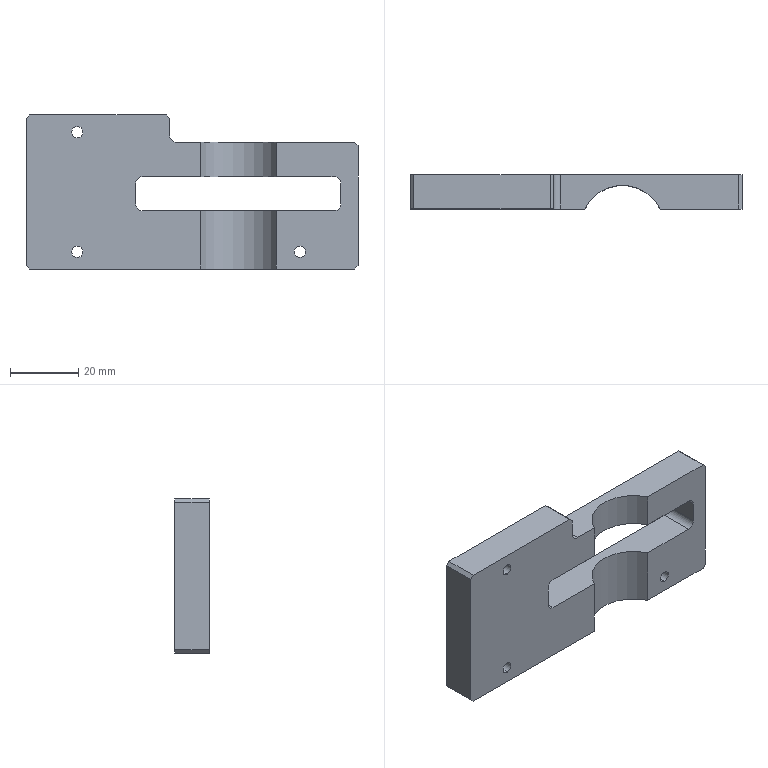Part | SolidWorks | features ICE 9, 3DProfileFeature 2, Fillet 2, HoleWzd 2, Chamfer 1, Extrusion 1 | 1 solid | 39 faces | box 97 x 10 x 45 mm | volume 29685 mm3 | plane 18 | cylinder 17 | cone 4 | commonest cylinder face diameters 3.3 x6 4 x5 4.2 x4 24.5 x2
STEP:
#1=CARTESIAN_POINT('',(-152.,0.,-19.15));
#2=VERTEX_POINT('',#1);
#3=CARTESIAN_POINT('',(-152.,0.,-15.85));
#4=VERTEX_POINT('',#3);
#5=CARTESIAN_POINT('',(-152.,0.,-17.5));
#6=DIRECTION('',(0.,1.,0.));
#7=DIRECTION('',(0.,0.,1.));
#8=AXIS2_PLACEMENT_3D('',#5,#6,#7);
#9=CIRCLE('',#8,1.65);
#10=EDGE_CURVE('',#2,#4,#9,.T.);
#11=ORIENTED_EDGE('',*,*,#10,.F.);
#12=CARTESIAN_POINT('',(-152.,10.,-19.15));
#13=VERTEX_POINT('',#12);
#14=CARTESIAN_POINT('',(-152.,10.,-19.15));
#15=DIRECTION('',(0.,1.,0.));
#16=VECTOR('',#15,1000.);
#17=LINE('',#14,#16);
#18=EDGE_CURVE('',#2,#13,#17,.T.);
#19=ORIENTED_EDGE('',*,*,#18,.T.);
#20=CARTESIAN_POINT('',(-152.,10.,-15.85));
#21=VERTEX_POINT('',#20);
#22=CARTESIAN_POINT('',(-152.,10.,-17.5));
#23=DIRECTION('',(0.,1.,0.));
#24=DIRECTION('',(0.,0.,1.));
#25=AXIS2_PLACEMENT_3D('',#22,#23,#24);
#26=CIRCLE('',#25,1.65);
#27=EDGE_CURVE('',#13,#21,#26,.T.);
#28=ORIENTED_EDGE('',*,*,#27,.T.);
#29=CARTESIAN_POINT('',(-152.,10.,-15.85));
#30=DIRECTION('',(0.,1.,0.));
#31=VECTOR('',#30,1000.);
#32=LINE('',#29,#31);
#33=EDGE_CURVE('',#4,#21,#32,.T.);
#34=ORIENTED_EDGE('',*,*,#33,.F.);
#35=EDGE_LOOP('',(#11,#19,#28,#34));
#36=FACE_OUTER_BOUND('',#35,.T.);
#37=CARTESIAN_POINT('',(-152.,10.,-17.5));
#38=DIRECTION('',(0.,1.,0.));
#39=DIRECTION('',(0.,0.,1.));
#40=AXIS2_PLACEMENT_3D('',#37,#38,#39);
#41=CYLINDRICAL_SURFACE('',#40,1.65);
#42=ADVANCED_FACE('',(#36),#41,.F.);
#43=CARTESIAN_POINT('',(-87.,0.,-19.15));
#44=VERTEX_POINT('',#43);
#45=CARTESIAN_POINT('',(-87.,0.,-15.85));
#46=VERTEX_POINT('',#45);
#47=CARTESIAN_POINT('',(-87.,0.,-17.5));
#48=DIRECTION('',(0.,1.,0.));
#49=DIRECTION('',(0.,0.,1.));
#50=AXIS2_PLACEMENT_3D('',#47,#48,#49);
#51=CIRCLE('',#50,1.65);
#52=EDGE_CURVE('',#44,#46,#51,.T.);
#53=ORIENTED_EDGE('',*,*,#52,.F.);
#54=CARTESIAN_POINT('',(-87.,10.,-19.15));
#55=VERTEX_POINT('',#54);
#56=CARTESIAN_POINT('',(-87.,10.,-19.15));
#57=DIRECTION('',(0.,1.,0.));
#58=VECTOR('',#57,1000.);
#59=LINE('',#56,#58);
#60=EDGE_CURVE('',#44,#55,#59,.T.);
#61=ORIENTED_EDGE('',*,*,#60,.T.);
#62=CARTESIAN_POINT('',(-87.,10.,-15.85));
#63=VERTEX_POINT('',#62);
#64=CARTESIAN_POINT('',(-87.,10.,-17.5));
#65=DIRECTION('',(0.,1.,0.));
#66=DIRECTION('',(0.,0.,1.));
#67=AXIS2_PLACEMENT_3D('',#64,#65,#66);
#68=CIRCLE('',#67,1.65);
#69=EDGE_CURVE('',#55,#63,#68,.T.);
#70=ORIENTED_EDGE('',*,*,#69,.T.);
#71=CARTESIAN_POINT('',(-87.,10.,-15.85));
#72=DIRECTION('',(0.,1.,0.));
#73=VECTOR('',#72,1000.);
#74=LINE('',#71,#73);
#75=EDGE_CURVE('',#46,#63,#74,.T.);
#76=ORIENTED_EDGE('',*,*,#75,.F.);
#77=EDGE_LOOP('',(#53,#61,#70,#76));
#78=FACE_OUTER_BOUND('',#77,.T.);
#79=CARTESIAN_POINT('',(-87.,10.,-17.5));
#80=DIRECTION('',(0.,1.,0.));
#81=DIRECTION('',(0.,0.,1.));
#82=AXIS2_PLACEMENT_3D('',#79,#80,#81);
#83=CYLINDRICAL_SURFACE('',#82,1.65);
#84=ADVANCED_FACE('',(#78),#83,.F.);
#85=CARTESIAN_POINT('',(-152.,0.,15.85));
#86=VERTEX_POINT('',#85);
#87=CARTESIAN_POINT('',(-152.,0.,19.15));
#88=VERTEX_POINT('',#87);
#89=CARTESIAN_POINT('',(-152.,0.,17.5));
#90=DIRECTION('',(0.,1.,0.));
#91=DIRECTION('',(0.,0.,1.));
#92=AXIS2_PLACEMENT_3D('',#89,#90,#91);
#93=CIRCLE('',#92,1.65);
#94=EDGE_CURVE('',#86,#88,#93,.T.);
#95=ORIENTED_EDGE('',*,*,#94,.F.);
#96=CARTESIAN_POINT('',(-152.,10.,15.85));
#97=VERTEX_POINT('',#96);
#98=CARTESIAN_POINT('',(-152.,10.,15.85));
#99=DIRECTION('',(0.,1.,0.));
#100=VECTOR('',#99,1000.);
#101=LINE('',#98,#100);
#102=EDGE_CURVE('',#86,#97,#101,.T.);
#103=ORIENTED_EDGE('',*,*,#102,.T.);
#104=CARTESIAN_POINT('',(-152.,10.,19.15));
#105=VERTEX_POINT('',#104);
#106=CARTESIAN_POINT('',(-152.,10.,17.5));
#107=DIRECTION('',(0.,1.,0.));
#108=DIRECTION('',(0.,0.,1.));
#109=AXIS2_PLACEMENT_3D('',#106,#107,#108);
#110=CIRCLE('',#109,1.65);
#111=EDGE_CURVE('',#97,#105,#110,.T.);
#112=ORIENTED_EDGE('',*,*,#111,.T.);
#113=CARTESIAN_POINT('',(-152.,10.,19.15));
#114=DIRECTION('',(0.,1.,0.));
#115=VECTOR('',#114,1000.);
#116=LINE('',#113,#115);
#117=EDGE_CURVE('',#88,#105,#116,.T.);
#118=ORIENTED_EDGE('',*,*,#117,.F.);
#119=EDGE_LOOP('',(#95,#103,#112,#118));
#120=FACE_OUTER_BOUND('',#119,.T.);
#121=CARTESIAN_POINT('',(-152.,10.,17.5));
#122=DIRECTION('',(0.,1.,0.));
#123=DIRECTION('',(0.,0.,1.));
#124=AXIS2_PLACEMENT_3D('',#121,#122,#123);
#125=CYLINDRICAL_SURFACE('',#124,1.65);
#126=ADVANCED_FACE('',(#120),#125,.F.);
#127=CARTESIAN_POINT('',(-156.9,5.,-10.1));
#128=VERTEX_POINT('',#127);
#129=CARTESIAN_POINT('',(-161.1,5.,-10.1));
#130=VERTEX_POINT('',#129);
#131=CARTESIAN_POINT('',(-159.,5.,-10.1));
#132=DIRECTION('',(0.,0.,-1.));
#133=DIRECTION('',(-1.,0.,0.));
#134=AXIS2_PLACEMENT_3D('',#131,#132,#133);
#135=CIRCLE('',#134,2.1);
#136=EDGE_CURVE('',#128,#130,#135,.T.);
#137=ORIENTED_EDGE('',*,*,#136,.F.);
#138=CARTESIAN_POINT('',(-156.9,5.,-22.5));
#139=VERTEX_POINT('',#138);
#140=CARTESIAN_POINT('',(-156.9,5.,-22.5));
#141=DIRECTION('',(0.,0.,-1.));
#142=VECTOR('',#141,1000.);
#143=LINE('',#140,#142);
#144=EDGE_CURVE('',#128,#139,#143,.T.);
#145=ORIENTED_EDGE('',*,*,#144,.T.);
#146=CARTESIAN_POINT('',(-161.1,5.,-22.5));
#147=VERTEX_POINT('',#146);
#148=CARTESIAN_POINT('',(-159.,5.,-22.5));
#149=DIRECTION('',(0.,0.,-1.));
#150=DIRECTION('',(-1.,0.,0.));
#151=AXIS2_PLACEMENT_3D('',#148,#149,#150);
#152=CIRCLE('',#151,2.1);
#153=EDGE_CURVE('',#139,#147,#152,.T.);
#154=ORIENTED_EDGE('',*,*,#153,.T.);
#155=CARTESIAN_POINT('',(-161.1,5.,-22.5));
#156=DIRECTION('',(0.,0.,-1.));
#157=VECTOR('',#156,1000.);
#158=LINE('',#155,#157);
#159=EDGE_CURVE('',#130,#147,#158,.T.);
#160=ORIENTED_EDGE('',*,*,#159,.F.);
#161=EDGE_LOOP('',(#137,#145,#154,#160));
#162=FACE_OUTER_BOUND('',#161,.T.);
#163=CARTESIAN_POINT('',(-159.,5.,-22.5));
#164=DIRECTION('',(0.,0.,-1.));
#165=DIRECTION('',(-1.,0.,0.));
#166=AXIS2_PLACEMENT_3D('',#163,#164,#165);
#167=CYLINDRICAL_SURFACE('',#166,2.1);
#168=ADVANCED_FACE('',(#162),#167,.F.);
#169=CARTESIAN_POINT('',(-159.,5.,-8.838));
#170=VERTEX_POINT('',#169);
#171=CARTESIAN_POINT('',(-161.1,5.,-10.1));
#172=DIRECTION('',(-0.8572,0.,-0.515));
#173=VECTOR('',#172,1000.);
#174=LINE('',#171,#173);
#175=EDGE_CURVE('',#170,#130,#174,.T.);
#176=ORIENTED_EDGE('',*,*,#175,.F.);
#177=CARTESIAN_POINT('',(-156.9,5.,-10.1));
#178=DIRECTION('',(0.8572,0.,-0.515));
#179=VECTOR('',#178,1000.);
#180=LINE('',#177,#179);
#181=EDGE_CURVE('',#170,#128,#180,.T.);
#182=ORIENTED_EDGE('',*,*,#181,.T.);
#183=ORIENTED_EDGE('',*,*,#136,.T.);
#184=EDGE_LOOP('',(#176,#182,#183));
#185=FACE_OUTER_BOUND('',#184,.T.);
#186=CARTESIAN_POINT('',(-159.,5.,-10.1));
#187=DIRECTION('',(0.,0.,-1.));
#188=DIRECTION('',(-1.,0.,0.));
#189=AXIS2_PLACEMENT_3D('',#186,#187,#188);
#190=CONICAL_SURFACE('',#189,2.1,1.03);
#191=ADVANCED_FACE('',(#185),#190,.F.);
#192=CARTESIAN_POINT('',(-78.9,5.,-10.1));
#193=VERTEX_POINT('',#192);
#194=CARTESIAN_POINT('',(-83.1,5.,-10.1));
#195=VERTEX_POINT('',#194);
#196=CARTESIAN_POINT('',(-81.,5.,-10.1));
#197=DIRECTION('',(0.,0.,-1.));
#198=DIRECTION('',(-1.,0.,0.));
#199=AXIS2_PLACEMENT_3D('',#196,#197,#198);
#200=CIRCLE('',#199,2.1);
#201=EDGE_CURVE('',#193,#195,#200,.T.);
#202=ORIENTED_EDGE('',*,*,#201,.F.);
#203=CARTESIAN_POINT('',(-78.9,5.,-22.5));
#204=VERTEX_POINT('',#203);
#205=CARTESIAN_POINT('',(-78.9,5.,-22.5));
#206=DIRECTION('',(0.,0.,-1.));
#207=VECTOR('',#206,1000.);
#208=LINE('',#205,#207);
#209=EDGE_CURVE('',#193,#204,#208,.T.);
#210=ORIENTED_EDGE('',*,*,#209,.T.);
#211=CARTESIAN_POINT('',(-83.1,5.,-22.5));
#212=VERTEX_POINT('',#211);
#213=CARTESIAN_POINT('',(-81.,5.,-22.5));
#214=DIRECTION('',(0.,0.,-1.));
#215=DIRECTION('',(-1.,0.,0.));
#216=AXIS2_PLACEMENT_3D('',#213,#214,#215);
#217=CIRCLE('',#216,2.1);
#218=EDGE_CURVE('',#204,#212,#217,.T.);
#219=ORIENTED_EDGE('',*,*,#218,.T.);
#220=CARTESIAN_POINT('',(-83.1,5.,-22.5));
#221=DIRECTION('',(0.,0.,-1.));
#222=VECTOR('',#221,1000.);
#223=LINE('',#220,#222);
#224=EDGE_CURVE('',#195,#212,#223,.T.);
#225=ORIENTED_EDGE('',*,*,#224,.F.);
#226=EDGE_LOOP('',(#202,#210,#219,#225));
#227=FACE_OUTER_BOUND('',#226,.T.);
#228=CARTESIAN_POINT('',(-81.,5.,-22.5));
#229=DIRECTION('',(0.,0.,-1.));
#230=DIRECTION('',(-1.,0.,0.));
#231=AXIS2_PLACEMENT_3D('',#228,#229,#230);
#232=CYLINDRICAL_SURFACE('',#231,2.1);
#233=ADVANCED_FACE('',(#227),#232,.F.);
#234=CARTESIAN_POINT('',(-81.,5.,-8.838));
#235=VERTEX_POINT('',#234);
#236=CARTESIAN_POINT('',(-83.1,5.,-10.1));
#237=DIRECTION('',(-0.8572,0.,-0.515));
#238=VECTOR('',#237,1000.);
#239=LINE('',#236,#238);
#240=EDGE_CURVE('',#235,#195,#239,.T.);
#241=ORIENTED_EDGE('',*,*,#240,.F.);
#242=CARTESIAN_POINT('',(-78.9,5.,-10.1));
#243=DIRECTION('',(0.8572,0.,-0.515));
#244=VECTOR('',#243,1000.);
#245=LINE('',#242,#244);
#246=EDGE_CURVE('',#235,#193,#245,.T.);
#247=ORIENTED_EDGE('',*,*,#246,.T.);
#248=ORIENTED_EDGE('',*,*,#201,.T.);
#249=EDGE_LOOP('',(#241,#247,#248));
#250=FACE_OUTER_BOUND('',#249,.T.);
#251=CARTESIAN_POINT('',(-81.,5.,-10.1));
#252=DIRECTION('',(0.,0.,-1.));
#253=DIRECTION('',(-1.,0.,0.));
#254=AXIS2_PLACEMENT_3D('',#251,#252,#253);
#255=CONICAL_SURFACE('',#254,2.1,1.03);
#256=ADVANCED_FACE('',(#250),#255,.F.);
#257=CARTESIAN_POINT('',(-152.,0.,-17.5));
#258=DIRECTION('',(0.,1.,0.));
#259=DIRECTION('',(0.,0.,1.));
#260=AXIS2_PLACEMENT_3D('',#257,#258,#259);
#261=CIRCLE('',#260,1.65);
#262=EDGE_CURVE('',#4,#2,#261,.T.);
#263=ORIENTED_EDGE('',*,*,#262,.T.);
#264=ORIENTED_EDGE('',*,*,#10,.T.);
#265=EDGE_LOOP('',(#263,#264));
#266=FACE_BOUND('',#265,.T.);
#267=CARTESIAN_POINT('',(-152.,0.,17.5));
#268=DIRECTION('',(0.,1.,0.));
#269=DIRECTION('',(0.,0.,1.));
#270=AXIS2_PLACEMENT_3D('',#267,#268,#269);
#271=CIRCLE('',#270,1.65);
#272=EDGE_CURVE('',#88,#86,#271,.T.);
#273=ORIENTED_EDGE('',*,*,#272,.T.);
#274=ORIENTED_EDGE('',*,*,#94,.T.);
#275=EDGE_LOOP('',(#273,#274));
#276=FACE_BOUND('',#275,.T.);
#277=CARTESIAN_POINT('',(-115.974,0.,14.5));
#278=VERTEX_POINT('',#277);
#279=CARTESIAN_POINT('',(-123.,0.,14.5));
#280=VERTEX_POINT('',#279);
#281=CARTESIAN_POINT('',(-70.,0.,14.5));
#282=DIRECTION('',(-1.,0.,0.));
#283=VECTOR('',#282,1000.);
#284=LINE('',#281,#283);
#285=EDGE_CURVE('',#278,#280,#284,.T.);
#286=ORIENTED_EDGE('',*,*,#285,.T.);
#287=CARTESIAN_POINT('',(-125.,0.,16.5));
#288=VERTEX_POINT('',#287);
#289=CARTESIAN_POINT('',(-123.,0.,16.5));
#290=DIRECTION('',(0.,1.,0.));
#291=DIRECTION('',(0.,0.,1.));
#292=AXIS2_PLACEMENT_3D('',#289,#290,#291);
#293=CIRCLE('',#292,2.);
#294=EDGE_CURVE('',#280,#288,#293,.T.);
#295=ORIENTED_EDGE('',*,*,#294,.T.);
#296=CARTESIAN_POINT('',(-125.,0.,21.5));
#297=VERTEX_POINT('',#296);
#298=CARTESIAN_POINT('',(-125.,0.,22.5));
#299=DIRECTION('',(0.,0.,1.));
#300=VECTOR('',#299,1000.);
#301=LINE('',#298,#300);
#302=EDGE_CURVE('',#288,#297,#301,.T.);
#303=ORIENTED_EDGE('',*,*,#302,.T.);
#304=CARTESIAN_POINT('',(-126.,0.,22.5));
#305=VERTEX_POINT('',#304);
#306=CARTESIAN_POINT('',(-126.,0.,22.5));
#307=DIRECTION('',(-0.7071,0.,0.7071));
#308=VECTOR('',#307,1000.);
#309=LINE('',#306,#308);
#310=EDGE_CURVE('',#297,#305,#309,.T.);
#311=ORIENTED_EDGE('',*,*,#310,.T.);
#312=CARTESIAN_POINT('',(-166.,0.,22.5));
#313=VERTEX_POINT('',#312);
#314=CARTESIAN_POINT('',(-145.,0.,22.5));
#315=DIRECTION('',(1.,0.,0.));
#316=VECTOR('',#315,1000.);
#317=LINE('',#314,#316);
#318=EDGE_CURVE('',#313,#305,#317,.T.);
#319=ORIENTED_EDGE('',*,*,#318,.F.);
#320=CARTESIAN_POINT('',(-167.,0.,21.5));
#321=VERTEX_POINT('',#320);
#322=CARTESIAN_POINT('',(-167.,0.,21.5));
#323=DIRECTION('',(-0.7071,0.,-0.7071));
#324=VECTOR('',#323,1000.);
#325=LINE('',#322,#324);
#326=EDGE_CURVE('',#313,#321,#325,.T.);
#327=ORIENTED_EDGE('',*,*,#326,.T.);
#328=CARTESIAN_POINT('',(-167.,0.,-21.5));
#329=VERTEX_POINT('',#328);
#330=CARTESIAN_POINT('',(-167.,0.,-22.5));
#331=DIRECTION('',(0.,0.,1.));
#332=VECTOR('',#331,1000.);
#333=LINE('',#330,#332);
#334=EDGE_CURVE('',#329,#321,#333,.T.);
#335=ORIENTED_EDGE('',*,*,#334,.F.);
#336=CARTESIAN_POINT('',(-166.,0.,-22.5));
#337=VERTEX_POINT('',#336);
#338=CARTESIAN_POINT('',(-167.,0.,-21.5));
#339=DIRECTION('',(0.7071,0.,-0.7071));
#340=VECTOR('',#339,1000.);
#341=LINE('',#338,#340);
#342=EDGE_CURVE('',#329,#337,#341,.T.);
#343=ORIENTED_EDGE('',*,*,#342,.T.);
#344=CARTESIAN_POINT('',(-115.974,0.,-22.5));
#345=VERTEX_POINT('',#344);
#346=CARTESIAN_POINT('',(-145.,0.,-22.5));
#347=DIRECTION('',(-1.,0.,0.));
#348=VECTOR('',#347,1000.);
#349=LINE('',#346,#348);
#350=EDGE_CURVE('',#345,#337,#349,.T.);
#351=ORIENTED_EDGE('',*,*,#350,.F.);
#352=CARTESIAN_POINT('',(-115.974,0.,-5.5));
#353=VERTEX_POINT('',#352);
#354=CARTESIAN_POINT('',(-115.974,0.,-22.5));
#355=DIRECTION('',(0.,0.,1.));
#356=VECTOR('',#355,1000.);
#357=LINE('',#354,#356);
#358=EDGE_CURVE('',#345,#353,#357,.T.);
#359=ORIENTED_EDGE('',*,*,#358,.T.);
#360=CARTESIAN_POINT('',(-133.,0.,-5.5));
#361=VERTEX_POINT('',#360);
#362=CARTESIAN_POINT('',(-135.,0.,-5.5));
#363=DIRECTION('',(-1.,0.,0.));
#364=VECTOR('',#363,1000.);
#365=LINE('',#362,#364);
#366=EDGE_CURVE('',#353,#361,#365,.T.);
#367=ORIENTED_EDGE('',*,*,#366,.T.);
#368=CARTESIAN_POINT('',(-135.,0.,-3.5));
#369=VERTEX_POINT('',#368);
#370=CARTESIAN_POINT('',(-133.,0.,-3.5));
#371=DIRECTION('',(0.,1.,0.));
#372=DIRECTION('',(0.,0.,1.));
#373=AXIS2_PLACEMENT_3D('',#370,#371,#372);
#374=CIRCLE('',#373,2.);
#375=EDGE_CURVE('',#361,#369,#374,.T.);
#376=ORIENTED_EDGE('',*,*,#375,.T.);
#377=CARTESIAN_POINT('',(-135.,0.,2.5));
#378=VERTEX_POINT('',#377);
#379=CARTESIAN_POINT('',(-135.,0.,-5.5));
#380=DIRECTION('',(0.,0.,1.));
#381=VECTOR('',#380,1000.);
#382=LINE('',#379,#381);
#383=EDGE_CURVE('',#369,#378,#382,.T.);
#384=ORIENTED_EDGE('',*,*,#383,.T.);
#385=CARTESIAN_POINT('',(-133.,0.,4.5));
#386=VERTEX_POINT('',#385);
#387=CARTESIAN_POINT('',(-133.,0.,2.5));
#388=DIRECTION('',(0.,1.,0.));
#389=DIRECTION('',(0.,0.,1.));
#390=AXIS2_PLACEMENT_3D('',#387,#388,#389);
#391=CIRCLE('',#390,2.);
#392=EDGE_CURVE('',#378,#386,#391,.T.);
#393=ORIENTED_EDGE('',*,*,#392,.T.);
#394=CARTESIAN_POINT('',(-115.974,0.,4.5));
#395=VERTEX_POINT('',#394);
#396=CARTESIAN_POINT('',(-135.,0.,4.5));
#397=DIRECTION('',(1.,0.,0.));
#398=VECTOR('',#397,1000.);
#399=LINE('',#396,#398);
#400=EDGE_CURVE('',#386,#395,#399,.T.);
#401=ORIENTED_EDGE('',*,*,#400,.T.);
#402=CARTESIAN_POINT('',(-115.974,0.,-22.5));
#403=DIRECTION('',(0.,0.,1.));
#404=VECTOR('',#403,1000.);
#405=LINE('',#402,#404);
#406=EDGE_CURVE('',#395,#278,#405,.T.);
#407=ORIENTED_EDGE('',*,*,#406,.T.);
#408=EDGE_LOOP('',(#286,#295,#303,#311,#319,#327,#335,#343,#351,#359,#367,#376,#384,#393,#401,#407));
#409=FACE_OUTER_BOUND('',#408,.T.);
#410=CARTESIAN_POINT('',(0.,0.,0.));
#411=DIRECTION('',(0.,1.,0.));
#412=DIRECTION('',(0.,0.,1.));
#413=AXIS2_PLACEMENT_3D('',#410,#411,#412);
#414=PLANE('',#413);
#415=ADVANCED_FACE('',(#266,#276,#409),#414,.F.);
#416=CARTESIAN_POINT('',(-159.,5.,-22.5));
#417=DIRECTION('',(0.,0.,-1.));
#418=DIRECTION('',(-1.,0.,0.));
#419=AXIS2_PLACEMENT_3D('',#416,#417,#418);
#420=CIRCLE('',#419,2.1);
#421=EDGE_CURVE('',#147,#139,#420,.T.);
#422=ORIENTED_EDGE('',*,*,#421,.F.);
#423=ORIENTED_EDGE('',*,*,#153,.F.);
#424=EDGE_LOOP('',(#422,#423));
#425=FACE_BOUND('',#424,.T.);
#426=CARTESIAN_POINT('',(-81.,5.,-22.5));
#427=DIRECTION('',(0.,0.,-1.));
#428=DIRECTION('',(-1.,0.,0.));
#429=AXIS2_PLACEMENT_3D('',#426,#427,#428);
#430=CIRCLE('',#429,2.1);
#431=EDGE_CURVE('',#212,#204,#430,.T.);
#432=ORIENTED_EDGE('',*,*,#431,.F.);
#433=ORIENTED_EDGE('',*,*,#218,.F.);
#434=EDGE_LOOP('',(#432,#433));
#435=FACE_BOUND('',#434,.T.);
#436=CARTESIAN_POINT('',(-71.,10.,-22.5));
#437=VERTEX_POINT('',#436);
#438=CARTESIAN_POINT('',(-166.,10.,-22.5));
#439=VERTEX_POINT('',#438);
#440=CARTESIAN_POINT('',(-145.,10.,-22.5));
#441=DIRECTION('',(-1.,0.,0.));
#442=VECTOR('',#441,1000.);
#443=LINE('',#440,#442);
#444=EDGE_CURVE('',#437,#439,#443,.T.);
#445=ORIENTED_EDGE('',*,*,#444,.F.);
#446=CARTESIAN_POINT('',(-71.,0.,-22.5));
#447=VERTEX_POINT('',#446);
#448=CARTESIAN_POINT('',(-71.,10.,-22.5));
#449=DIRECTION('',(0.,-1.,0.));
#450=VECTOR('',#449,1000.);
#451=LINE('',#448,#450);
#452=EDGE_CURVE('',#437,#447,#451,.T.);
#453=ORIENTED_EDGE('',*,*,#452,.T.);
#454=CARTESIAN_POINT('',(-93.886,0.,-22.5));
#455=VERTEX_POINT('',#454);
#456=CARTESIAN_POINT('',(-145.,0.,-22.5));
#457=DIRECTION('',(-1.,0.,0.));
#458=VECTOR('',#457,1000.);
#459=LINE('',#456,#458);
#460=EDGE_CURVE('',#447,#455,#459,.T.);
#461=ORIENTED_EDGE('',*,*,#460,.T.);
#462=CARTESIAN_POINT('',(-104.93,-5.3,-22.5));
#463=DIRECTION('',(0.,0.,1.));
#464=DIRECTION('',(1.,0.,0.));
#465=AXIS2_PLACEMENT_3D('',#462,#463,#464);
#466=CIRCLE('',#465,12.25);
#467=EDGE_CURVE('',#455,#345,#466,.T.);
#468=ORIENTED_EDGE('',*,*,#467,.T.);
#469=ORIENTED_EDGE('',*,*,#350,.T.);
#470=CARTESIAN_POINT('',(-166.,10.,-22.5));
#471=DIRECTION('',(0.,1.,0.));
#472=VECTOR('',#471,1000.);
#473=LINE('',#470,#472);
#474=EDGE_CURVE('',#337,#439,#473,.T.);
#475=ORIENTED_EDGE('',*,*,#474,.T.);
#476=EDGE_LOOP('',(#445,#453,#461,#468,#469,#475));
#477=FACE_OUTER_BOUND('',#476,.T.);
#478=CARTESIAN_POINT('',(-145.,10.,-22.5));
#479=DIRECTION('',(0.,0.,1.));
#480=DIRECTION('',(1.,0.,0.));
#481=AXIS2_PLACEMENT_3D('',#478,#479,#480);
#482=PLANE('',#481);
#483=ADVANCED_FACE('',(#425,#435,#477),#482,.F.);
#484=ORIENTED_EDGE('',*,*,#318,.T.);
#485=CARTESIAN_POINT('',(-126.,10.,22.5));
#486=VERTEX_POINT('',#485);
#487=CARTESIAN_POINT('',(-126.,10.,22.5));
#488=DIRECTION('',(0.,1.,0.));
#489=VECTOR('',#488,1000.);
#490=LINE('',#487,#489);
#491=EDGE_CURVE('',#305,#486,#490,.T.);
#492=ORIENTED_EDGE('',*,*,#491,.T.);
#493=CARTESIAN_POINT('',(-166.,10.,22.5));
#494=VERTEX_POINT('',#493);
#495=CARTESIAN_POINT('',(-145.,10.,22.5));
#496=DIRECTION('',(1.,0.,0.));
#497=VECTOR('',#496,1000.);
#498=LINE('',#495,#497);
#499=EDGE_CURVE('',#494,#486,#498,.T.);
#500=ORIENTED_EDGE('',*,*,#499,.F.);
#501=CARTESIAN_POINT('',(-166.,0.,22.5));
#502=DIRECTION('',(0.,-1.,0.));
#503=VECTOR('',#502,1000.);
#504=LINE('',#501,#503);
#505=EDGE_CURVE('',#494,#313,#504,.T.);
#506=ORIENTED_EDGE('',*,*,#505,.T.);
#507=EDGE_LOOP('',(#484,#492,#500,#506));
#508=FACE_OUTER_BOUND('',#507,.T.);
#509=CARTESIAN_POINT('',(-145.,10.,22.5));
#510=DIRECTION('',(0.,0.,-1.));
#511=DIRECTION('',(-1.,0.,0.));
#512=AXIS2_PLACEMENT_3D('',#509,#510,#511);
#513=PLANE('',#512);
#514=ADVANCED_FACE('',(#508),#513,.F.);
#515=CARTESIAN_POINT('',(-152.,10.,-17.5));
#516=DIRECTION('',(0.,1.,0.));
#517=DIRECTION('',(0.,0.,1.));
#518=AXIS2_PLACEMENT_3D('',#515,#516,#517);
#519=CIRCLE('',#518,1.65);
#520=EDGE_CURVE('',#21,#13,#519,.T.);
#521=ORIENTED_EDGE('',*,*,#520,.F.);
#522=ORIENTED_EDGE('',*,*,#27,.F.);
#523=EDGE_LOOP('',(#521,#522));
#524=FACE_BOUND('',#523,.T.);
#525=CARTESIAN_POINT('',(-87.,10.,-17.5));
#526=DIRECTION('',(0.,1.,0.));
#527=DIRECTION('',(0.,0.,1.));
#528=AXIS2_PLACEMENT_3D('',#525,#526,#527);
#529=CIRCLE('',#528,1.65);
#530=EDGE_CURVE('',#63,#55,#529,.T.);
#531=ORIENTED_EDGE('',*,*,#530,.F.);
#532=ORIENTED_EDGE('',*,*,#69,.F.);
#533=EDGE_LOOP('',(#531,#532));
#534=FACE_BOUND('',#533,.T.);
#535=CARTESIAN_POINT('',(-152.,10.,17.5));
#536=DIRECTION('',(0.,1.,0.));
#537=DIRECTION('',(0.,0.,1.));
#538=AXIS2_PLACEMENT_3D('',#535,#536,#537);
#539=CIRCLE('',#538,1.65);
#540=EDGE_CURVE('',#105,#97,#539,.T.);
#541=ORIENTED_EDGE('',*,*,#540,.F.);
#542=ORIENTED_EDGE('',*,*,#111,.F.);
#543=EDGE_LOOP('',(#541,#542));
#544=FACE_BOUND('',#543,.T.);
#545=ORIENTED_EDGE('',*,*,#499,.T.);
#546=CARTESIAN_POINT('',(-125.,10.,21.5));
#547=VERTEX_POINT('',#546);
#548=CARTESIAN_POINT('',(-51.75,10.,-51.75));
#549=DIRECTION('',(0.7071,0.,-0.7071));
#550=VECTOR('',#549,1000.);
#551=LINE('',#548,#550);
#552=EDGE_CURVE('',#486,#547,#551,.T.);
#553=ORIENTED_EDGE('',*,*,#552,.T.);
#554=CARTESIAN_POINT('',(-125.,10.,16.5));
#555=VERTEX_POINT('',#554);
#556=CARTESIAN_POINT('',(-125.,10.,22.5));
#557=DIRECTION('',(0.,0.,1.));
#558=VECTOR('',#557,1000.);
#559=LINE('',#556,#558);
#560=EDGE_CURVE('',#555,#547,#559,.T.);
#561=ORIENTED_EDGE('',*,*,#560,.F.);
#562=CARTESIAN_POINT('',(-123.,10.,14.5));
#563=VERTEX_POINT('',#562);
#564=CARTESIAN_POINT('',(-123.,10.,16.5));
#565=DIRECTION('',(0.,-1.,0.));
#566=DIRECTION('',(0.,0.,1.));
#567=AXIS2_PLACEMENT_3D('',#564,#565,#566);
#568=CIRCLE('',#567,2.);
#569=EDGE_CURVE('',#555,#563,#568,.T.);
#570=ORIENTED_EDGE('',*,*,#569,.T.);
#571=CARTESIAN_POINT('',(-71.,10.,14.5));
#572=VERTEX_POINT('',#571);
#573=CARTESIAN_POINT('',(-70.,10.,14.5));
#574=DIRECTION('',(-1.,0.,0.));
#575=VECTOR('',#574,1000.);
#576=LINE('',#573,#575);
#577=EDGE_CURVE('',#572,#563,#576,.T.);
#578=ORIENTED_EDGE('',*,*,#577,.F.);
#579=CARTESIAN_POINT('',(-70.,10.,13.5));
#580=VERTEX_POINT('',#579);
#581=CARTESIAN_POINT('',(-28.25,10.,-28.25));
#582=DIRECTION('',(0.7071,0.,-0.7071));
#583=VECTOR('',#582,1000.);
#584=LINE('',#581,#583);
#585=EDGE_CURVE('',#572,#580,#584,.T.);
#586=ORIENTED_EDGE('',*,*,#585,.T.);
#587=CARTESIAN_POINT('',(-70.,10.,-21.5));
#588=VERTEX_POINT('',#587);
#589=CARTESIAN_POINT('',(-70.,10.,0.));
#590=DIRECTION('',(0.,0.,1.));
#591=VECTOR('',#590,1000.);
#592=LINE('',#589,#591);
#593=EDGE_CURVE('',#588,#580,#592,.T.);
#594=ORIENTED_EDGE('',*,*,#593,.F.);
#595=CARTESIAN_POINT('',(-24.25,10.,24.25));
#596=DIRECTION('',(-0.7071,0.,-0.7071));
#597=VECTOR('',#596,1000.);
#598=LINE('',#595,#597);
#599=EDGE_CURVE('',#588,#437,#598,.T.);
#600=ORIENTED_EDGE('',*,*,#599,.T.);
#601=ORIENTED_EDGE('',*,*,#444,.T.);
#602=CARTESIAN_POINT('',(-167.,10.,-21.5));
#603=VERTEX_POINT('',#602);
#604=CARTESIAN_POINT('',(-94.25,10.,-94.25));
#605=DIRECTION('',(-0.7071,0.,0.7071));
#606=VECTOR('',#605,1000.);
#607=LINE('',#604,#606);
#608=EDGE_CURVE('',#439,#603,#607,.T.);
#609=ORIENTED_EDGE('',*,*,#608,.T.);
#610=CARTESIAN_POINT('',(-167.,10.,21.5));
#611=VERTEX_POINT('',#610);
#612=CARTESIAN_POINT('',(-167.,10.,-22.5));
#613=DIRECTION('',(0.,0.,-1.));
#614=VECTOR('',#613,1000.);
#615=LINE('',#612,#614);
#616=EDGE_CURVE('',#611,#603,#615,.T.);
#617=ORIENTED_EDGE('',*,*,#616,.F.);
#618=CARTESIAN_POINT('',(-94.25,10.,94.25));
#619=DIRECTION('',(0.7071,0.,0.7071));
#620=VECTOR('',#619,1000.);
#621=LINE('',#618,#620);
#622=EDGE_CURVE('',#611,#494,#621,.T.);
#623=ORIENTED_EDGE('',*,*,#622,.T.);
#624=EDGE_LOOP('',(#545,#553,#561,#570,#578,#586,#594,#600,#601,#609,#617,#623));
#625=FACE_OUTER_BOUND('',#624,.T.);
#626=CARTESIAN_POINT('',(-75.,10.,2.5));
#627=VERTEX_POINT('',#626);
#628=CARTESIAN_POINT('',(-75.,10.,-3.5));
#629=VERTEX_POINT('',#628);
#630=CARTESIAN_POINT('',(-75.,10.,-5.5));
#631=DIRECTION('',(0.,0.,-1.));
#632=VECTOR('',#631,1000.);
#633=LINE('',#630,#632);
#634=EDGE_CURVE('',#627,#629,#633,.T.);
#635=ORIENTED_EDGE('',*,*,#634,.F.);
#636=CARTESIAN_POINT('',(-77.,10.,4.5));
#637=VERTEX_POINT('',#636);
#638=CARTESIAN_POINT('',(-77.,10.,2.5));
#639=DIRECTION('',(0.,-1.,0.));
#640=DIRECTION('',(0.,0.,1.));
#641=AXIS2_PLACEMENT_3D('',#638,#639,#640);
#642=CIRCLE('',#641,2.);
#643=EDGE_CURVE('',#627,#637,#642,.T.);
#644=ORIENTED_EDGE('',*,*,#643,.T.);
#645=CARTESIAN_POINT('',(-133.,10.,4.5));
#646=VERTEX_POINT('',#645);
#647=CARTESIAN_POINT('',(-135.,10.,4.5));
#648=DIRECTION('',(1.,0.,0.));
#649=VECTOR('',#648,1000.);
#650=LINE('',#647,#649);
#651=EDGE_CURVE('',#646,#637,#650,.T.);
#652=ORIENTED_EDGE('',*,*,#651,.F.);
#653=CARTESIAN_POINT('',(-135.,10.,2.5));
#654=VERTEX_POINT('',#653);
#655=CARTESIAN_POINT('',(-133.,10.,2.5));
#656=DIRECTION('',(0.,-1.,0.));
#657=DIRECTION('',(0.,0.,1.));
#658=AXIS2_PLACEMENT_3D('',#655,#656,#657);
#659=CIRCLE('',#658,2.);
#660=EDGE_CURVE('',#646,#654,#659,.T.);
#661=ORIENTED_EDGE('',*,*,#660,.T.);
#662=CARTESIAN_POINT('',(-135.,10.,-3.5));
#663=VERTEX_POINT('',#662);
#664=CARTESIAN_POINT('',(-135.,10.,-5.5));
#665=DIRECTION('',(0.,0.,1.));
#666=VECTOR('',#665,1000.);
#667=LINE('',#664,#666);
#668=EDGE_CURVE('',#663,#654,#667,.T.);
#669=ORIENTED_EDGE('',*,*,#668,.F.);
#670=CARTESIAN_POINT('',(-133.,10.,-5.5));
#671=VERTEX_POINT('',#670);
#672=CARTESIAN_POINT('',(-133.,10.,-3.5));
#673=DIRECTION('',(0.,-1.,0.));
#674=DIRECTION('',(0.,0.,1.));
#675=AXIS2_PLACEMENT_3D('',#672,#673,#674);
#676=CIRCLE('',#675,2.);
#677=EDGE_CURVE('',#663,#671,#676,.T.);
#678=ORIENTED_EDGE('',*,*,#677,.T.);
#679=CARTESIAN_POINT('',(-77.,10.,-5.5));
#680=VERTEX_POINT('',#679);
#681=CARTESIAN_POINT('',(-135.,10.,-5.5));
#682=DIRECTION('',(-1.,0.,0.));
#683=VECTOR('',#682,1000.);
#684=LINE('',#681,#683);
#685=EDGE_CURVE('',#680,#671,#684,.T.);
#686=ORIENTED_EDGE('',*,*,#685,.F.);
#687=CARTESIAN_POINT('',(-77.,10.,-3.5));
#688=DIRECTION('',(0.,-1.,0.));
#689=DIRECTION('',(0.,0.,1.));
#690=AXIS2_PLACEMENT_3D('',#687,#688,#689);
#691=CIRCLE('',#690,2.);
#692=EDGE_CURVE('',#680,#629,#691,.T.);
#693=ORIENTED_EDGE('',*,*,#692,.T.);
#694=EDGE_LOOP('',(#635,#644,#652,#661,#669,#678,#686,#693));
#695=FACE_BOUND('',#694,.T.);
#696=CARTESIAN_POINT('',(0.,10.,0.));
#697=DIRECTION('',(0.,1.,0.));
#698=DIRECTION('',(0.,0.,1.));
#699=AXIS2_PLACEMENT_3D('',#696,#697,#698);
#700=PLANE('',#699);
#701=ADVANCED_FACE('',(#524,#534,#544,#625,#695),#700,.T.);
#702=CARTESIAN_POINT('',(-87.,0.,-17.5));
#703=DIRECTION('',(0.,1.,0.));
#704=DIRECTION('',(0.,0.,1.));
#705=AXIS2_PLACEMENT_3D('',#702,#703,#704);
#706=CIRCLE('',#705,1.65);
#707=EDGE_CURVE('',#46,#44,#706,.T.);
#708=ORIENTED_EDGE('',*,*,#707,.T.);
#709=ORIENTED_EDGE('',*,*,#52,.T.);
#710=EDGE_LOOP('',(#708,#709));
#711=FACE_BOUND('',#710,.T.);
#712=ORIENTED_EDGE('',*,*,#460,.F.);
#713=CARTESIAN_POINT('',(-70.,0.,-21.5));
#714=VERTEX_POINT('',#713);
#715=CARTESIAN_POINT('',(-70.,0.,-21.5));
#716=DIRECTION('',(0.7071,0.,0.7071));
#717=VECTOR('',#716,1000.);
#718=LINE('',#715,#717);
#719=EDGE_CURVE('',#447,#714,#718,.T.);
#720=ORIENTED_EDGE('',*,*,#719,.T.);
#721=CARTESIAN_POINT('',(-70.,0.,13.5));
#722=VERTEX_POINT('',#721);
#723=CARTESIAN_POINT('',(-70.,0.,0.));
#724=DIRECTION('',(0.,0.,1.));
#725=VECTOR('',#724,1000.);
#726=LINE('',#723,#725);
#727=EDGE_CURVE('',#714,#722,#726,.T.);
#728=ORIENTED_EDGE('',*,*,#727,.T.);
#729=CARTESIAN_POINT('',(-71.,0.,14.5));
#730=VERTEX_POINT('',#729);
#731=CARTESIAN_POINT('',(-71.,0.,14.5));
#732=DIRECTION('',(-0.7071,0.,0.7071));
#733=VECTOR('',#732,1000.);
#734=LINE('',#731,#733);
#735=EDGE_CURVE('',#722,#730,#734,.T.);
#736=ORIENTED_EDGE('',*,*,#735,.T.);
#737=CARTESIAN_POINT('',(-93.886,0.,14.5));
#738=VERTEX_POINT('',#737);
#739=CARTESIAN_POINT('',(-70.,0.,14.5));
#740=DIRECTION('',(-1.,0.,0.));
#741=VECTOR('',#740,1000.);
#742=LINE('',#739,#741);
#743=EDGE_CURVE('',#730,#738,#742,.T.);
#744=ORIENTED_EDGE('',*,*,#743,.T.);
#745=CARTESIAN_POINT('',(-93.886,0.,4.5));
#746=VERTEX_POINT('',#745);
#747=CARTESIAN_POINT('',(-93.886,0.,-22.5));
#748=DIRECTION('',(0.,0.,-1.));
#749=VECTOR('',#748,1000.);
#750=LINE('',#747,#749);
#751=EDGE_CURVE('',#738,#746,#750,.T.);
#752=ORIENTED_EDGE('',*,*,#751,.T.);
#753=CARTESIAN_POINT('',(-77.,0.,4.5));
#754=VERTEX_POINT('',#753);
#755=CARTESIAN_POINT('',(-135.,0.,4.5));
#756=DIRECTION('',(1.,0.,0.));
#757=VECTOR('',#756,1000.);
#758=LINE('',#755,#757);
#759=EDGE_CURVE('',#746,#754,#758,.T.);
#760=ORIENTED_EDGE('',*,*,#759,.T.);
#761=CARTESIAN_POINT('',(-75.,0.,2.5));
#762=VERTEX_POINT('',#761);
#763=CARTESIAN_POINT('',(-77.,0.,2.5));
#764=DIRECTION('',(0.,1.,0.));
#765=DIRECTION('',(0.,0.,1.));
#766=AXIS2_PLACEMENT_3D('',#763,#764,#765);
#767=CIRCLE('',#766,2.);
#768=EDGE_CURVE('',#754,#762,#767,.T.);
#769=ORIENTED_EDGE('',*,*,#768,.T.);
#770=CARTESIAN_POINT('',(-75.,0.,-3.5));
#771=VERTEX_POINT('',#770);
#772=CARTESIAN_POINT('',(-75.,0.,-5.5));
#773=DIRECTION('',(0.,0.,-1.));
#774=VECTOR('',#773,1000.);
#775=LINE('',#772,#774);
#776=EDGE_CURVE('',#762,#771,#775,.T.);
#777=ORIENTED_EDGE('',*,*,#776,.T.);
#778=CARTESIAN_POINT('',(-77.,0.,-5.5));
#779=VERTEX_POINT('',#778);
#780=CARTESIAN_POINT('',(-77.,0.,-3.5));
#781=DIRECTION('',(0.,1.,0.));
#782=DIRECTION('',(0.,0.,1.));
#783=AXIS2_PLACEMENT_3D('',#780,#781,#782);
#784=CIRCLE('',#783,2.);
#785=EDGE_CURVE('',#771,#779,#784,.T.);
#786=ORIENTED_EDGE('',*,*,#785,.T.);
#787=CARTESIAN_POINT('',(-93.886,0.,-5.5));
#788=VERTEX_POINT('',#787);
#789=CARTESIAN_POINT('',(-135.,0.,-5.5));
#790=DIRECTION('',(-1.,0.,0.));
#791=VECTOR('',#790,1000.);
#792=LINE('',#789,#791);
#793=EDGE_CURVE('',#779,#788,#792,.T.);
#794=ORIENTED_EDGE('',*,*,#793,.T.);
#795=CARTESIAN_POINT('',(-93.886,0.,-22.5));
#796=DIRECTION('',(0.,0.,-1.));
#797=VECTOR('',#796,1000.);
#798=LINE('',#795,#797);
#799=EDGE_CURVE('',#788,#455,#798,.T.);
#800=ORIENTED_EDGE('',*,*,#799,.T.);
#801=EDGE_LOOP('',(#712,#720,#728,#736,#744,#752,#760,#769,#777,#786,#794,#800));
#802=FACE_OUTER_BOUND('',#801,.T.);
#803=CARTESIAN_POINT('',(0.,0.,0.));
#804=DIRECTION('',(0.,1.,0.));
#805=DIRECTION('',(0.,0.,1.));
#806=AXIS2_PLACEMENT_3D('',#803,#804,#805);
#807=PLANE('',#806);
#808=ADVANCED_FACE('',(#711,#802),#807,.F.);
#809=ORIENTED_EDGE('',*,*,#634,.T.);
#810=CARTESIAN_POINT('',(-75.,0.,-3.5));
#811=DIRECTION('',(0.,-1.,0.));
#812=VECTOR('',#811,1000.);
#813=LINE('',#810,#812);
#814=EDGE_CURVE('',#629,#771,#813,.T.);
#815=ORIENTED_EDGE('',*,*,#814,.T.);
#816=ORIENTED_EDGE('',*,*,#776,.F.);
#817=CARTESIAN_POINT('',(-75.,10.,2.5));
#818=DIRECTION('',(0.,1.,0.));
#819=VECTOR('',#818,1000.);
#820=LINE('',#817,#819);
#821=EDGE_CURVE('',#762,#627,#820,.T.);
#822=ORIENTED_EDGE('',*,*,#821,.T.);
#823=EDGE_LOOP('',(#809,#815,#816,#822));
#824=FACE_OUTER_BOUND('',#823,.T.);
#825=CARTESIAN_POINT('',(-75.,0.,-5.5));
#826=DIRECTION('',(1.,0.,0.));
#827=DIRECTION('',(0.,0.,-1.));
#828=AXIS2_PLACEMENT_3D('',#825,#826,#827);
#829=PLANE('',#828);
#830=ADVANCED_FACE('',(#824),#829,.F.);
#831=ORIENTED_EDGE('',*,*,#651,.T.);
#832=CARTESIAN_POINT('',(-77.,0.,4.5));
#833=DIRECTION('',(0.,-1.,0.));
#834=VECTOR('',#833,1000.);
#835=LINE('',#832,#834);
#836=EDGE_CURVE('',#637,#754,#835,.T.);
#837=ORIENTED_EDGE('',*,*,#836,.T.);
#838=ORIENTED_EDGE('',*,*,#759,.F.);
#839=CARTESIAN_POINT('',(-104.93,-5.3,4.5));
#840=DIRECTION('',(0.,0.,1.));
#841=DIRECTION('',(1.,0.,0.));
#842=AXIS2_PLACEMENT_3D('',#839,#840,#841);
#843=CIRCLE('',#842,12.25);
#844=EDGE_CURVE('',#746,#395,#843,.T.);
#845=ORIENTED_EDGE('',*,*,#844,.T.);
#846=ORIENTED_EDGE('',*,*,#400,.F.);
#847=CARTESIAN_POINT('',(-133.,10.,4.5));
#848=DIRECTION('',(0.,1.,0.));
#849=VECTOR('',#848,1000.);
#850=LINE('',#847,#849);
#851=EDGE_CURVE('',#386,#646,#850,.T.);
#852=ORIENTED_EDGE('',*,*,#851,.T.);
#853=EDGE_LOOP('',(#831,#837,#838,#845,#846,#852));
#854=FACE_OUTER_BOUND('',#853,.T.);
#855=CARTESIAN_POINT('',(-135.,0.,4.5));
#856=DIRECTION('',(0.,0.,1.));
#857=DIRECTION('',(1.,0.,0.));
#858=AXIS2_PLACEMENT_3D('',#855,#856,#857);
#859=PLANE('',#858);
#860=ADVANCED_FACE('',(#854),#859,.F.);
#861=ORIENTED_EDGE('',*,*,#383,.F.);
#862=CARTESIAN_POINT('',(-135.,10.,-3.5));
#863=DIRECTION('',(0.,1.,0.));
#864=VECTOR('',#863,1000.);
#865=LINE('',#862,#864);
#866=EDGE_CURVE('',#369,#663,#865,.T.);
#867=ORIENTED_EDGE('',*,*,#866,.T.);
#868=ORIENTED_EDGE('',*,*,#668,.T.);
#869=CARTESIAN_POINT('',(-135.,0.,2.5));
#870=DIRECTION('',(0.,-1.,0.));
#871=VECTOR('',#870,1000.);
#872=LINE('',#869,#871);
#873=EDGE_CURVE('',#654,#378,#872,.T.);
#874=ORIENTED_EDGE('',*,*,#873,.T.);
#875=EDGE_LOOP('',(#861,#867,#868,#874));
#876=FACE_OUTER_BOUND('',#875,.T.);
#877=CARTESIAN_POINT('',(-135.,0.,-5.5));
#878=DIRECTION('',(-1.,0.,0.));
#879=DIRECTION('',(0.,0.,1.));
#880=AXIS2_PLACEMENT_3D('',#877,#878,#879);
#881=PLANE('',#880);
#882=ADVANCED_FACE('',(#876),#881,.F.);
#883=ORIENTED_EDGE('',*,*,#793,.F.);
#884=CARTESIAN_POINT('',(-77.,10.,-5.5));
#885=DIRECTION('',(0.,1.,0.));
#886=VECTOR('',#885,1000.);
#887=LINE('',#884,#886);
#888=EDGE_CURVE('',#779,#680,#887,.T.);
#889=ORIENTED_EDGE('',*,*,#888,.T.);
#890=ORIENTED_EDGE('',*,*,#685,.T.);
#891=CARTESIAN_POINT('',(-133.,0.,-5.5));
#892=DIRECTION('',(0.,-1.,0.));
#893=VECTOR('',#892,1000.);
#894=LINE('',#891,#893);
#895=EDGE_CURVE('',#671,#361,#894,.T.);
#896=ORIENTED_EDGE('',*,*,#895,.T.);
#897=ORIENTED_EDGE('',*,*,#366,.F.);
#898=CARTESIAN_POINT('',(-104.93,-5.3,-5.5));
#899=DIRECTION('',(0.,0.,-1.));
#900=DIRECTION('',(-1.,0.,0.));
#901=AXIS2_PLACEMENT_3D('',#898,#899,#900);
#902=CIRCLE('',#901,12.25);
#903=EDGE_CURVE('',#353,#788,#902,.T.);
#904=ORIENTED_EDGE('',*,*,#903,.T.);
#905=EDGE_LOOP('',(#883,#889,#890,#896,#897,#904));
#906=FACE_OUTER_BOUND('',#905,.T.);
#907=CARTESIAN_POINT('',(-135.,0.,-5.5));
#908=DIRECTION('',(0.,0.,-1.));
#909=DIRECTION('',(-1.,0.,0.));
#910=AXIS2_PLACEMENT_3D('',#907,#908,#909);
#911=PLANE('',#910);
#912=ADVANCED_FACE('',(#906),#911,.F.);
#913=ORIENTED_EDGE('',*,*,#616,.T.);
#914=CARTESIAN_POINT('',(-167.,0.,-21.5));
#915=DIRECTION('',(0.,-1.,0.));
#916=VECTOR('',#915,1000.);
#917=LINE('',#914,#916);
#918=EDGE_CURVE('',#603,#329,#917,.T.);
#919=ORIENTED_EDGE('',*,*,#918,.T.);
#920=ORIENTED_EDGE('',*,*,#334,.T.);
#921=CARTESIAN_POINT('',(-167.,10.,21.5));
#922=DIRECTION('',(0.,1.,0.));
#923=VECTOR('',#922,1000.);
#924=LINE('',#921,#923);
#925=EDGE_CURVE('',#321,#611,#924,.T.);
#926=ORIENTED_EDGE('',*,*,#925,.T.);
#927=EDGE_LOOP('',(#913,#919,#920,#926));
#928=FACE_OUTER_BOUND('',#927,.T.);
#929=CARTESIAN_POINT('',(-167.,0.,0.));
#930=DIRECTION('',(-1.,0.,0.));
#931=DIRECTION('',(0.,0.,1.));
#932=AXIS2_PLACEMENT_3D('',#929,#930,#931);
#933=PLANE('',#932);
#934=ADVANCED_FACE('',(#928),#933,.T.);
#935=ORIENTED_EDGE('',*,*,#727,.F.);
#936=CARTESIAN_POINT('',(-70.,27.,-21.5));
#937=DIRECTION('',(0.,1.,0.));
#938=VECTOR('',#937,1000.);
#939=LINE('',#936,#938);
#940=EDGE_CURVE('',#714,#588,#939,.T.);
#941=ORIENTED_EDGE('',*,*,#940,.T.);
#942=ORIENTED_EDGE('',*,*,#593,.T.);
#943=CARTESIAN_POINT('',(-70.,27.,13.5));
#944=DIRECTION('',(0.,-1.,0.));
#945=VECTOR('',#944,1000.);
#946=LINE('',#943,#945);
#947=EDGE_CURVE('',#580,#722,#946,.T.);
#948=ORIENTED_EDGE('',*,*,#947,.T.);
#949=EDGE_LOOP('',(#935,#941,#942,#948));
#950=FACE_OUTER_BOUND('',#949,.T.);
#951=CARTESIAN_POINT('',(-70.,27.,12.));
#952=DIRECTION('',(-1.,0.,0.));
#953=DIRECTION('',(0.,0.,1.));
#954=AXIS2_PLACEMENT_3D('',#951,#952,#953);
#955=PLANE('',#954);
#956=ADVANCED_FACE('',(#950),#955,.F.);
#957=ORIENTED_EDGE('',*,*,#246,.F.);
#958=ORIENTED_EDGE('',*,*,#240,.T.);
#959=CARTESIAN_POINT('',(-81.,5.,-10.1));
#960=DIRECTION('',(0.,0.,-1.));
#961=DIRECTION('',(-1.,0.,0.));
#962=AXIS2_PLACEMENT_3D('',#959,#960,#961);
#963=CIRCLE('',#962,2.1);
#964=EDGE_CURVE('',#195,#193,#963,.T.);
#965=ORIENTED_EDGE('',*,*,#964,.T.);
#966=EDGE_LOOP('',(#957,#958,#965));
#967=FACE_OUTER_BOUND('',#966,.T.);
#968=CARTESIAN_POINT('',(-81.,5.,-10.1));
#969=DIRECTION('',(0.,0.,-1.));
#970=DIRECTION('',(-1.,0.,0.));
#971=AXIS2_PLACEMENT_3D('',#968,#969,#970);
#972=CONICAL_SURFACE('',#971,2.1,1.03);
#973=ADVANCED_FACE('',(#967),#972,.F.);
#974=ORIENTED_EDGE('',*,*,#209,.F.);
#975=ORIENTED_EDGE('',*,*,#964,.F.);
#976=ORIENTED_EDGE('',*,*,#224,.T.);
#977=ORIENTED_EDGE('',*,*,#431,.T.);
#978=EDGE_LOOP('',(#974,#975,#976,#977));
#979=FACE_OUTER_BOUND('',#978,.T.);
#980=CARTESIAN_POINT('',(-81.,5.,-22.5));
#981=DIRECTION('',(0.,0.,-1.));
#982=DIRECTION('',(-1.,0.,0.));
#983=AXIS2_PLACEMENT_3D('',#980,#981,#982);
#984=CYLINDRICAL_SURFACE('',#983,2.1);
#985=ADVANCED_FACE('',(#979),#984,.F.);
#986=ORIENTED_EDGE('',*,*,#181,.F.);
#987=ORIENTED_EDGE('',*,*,#175,.T.);
#988=CARTESIAN_POINT('',(-159.,5.,-10.1));
#989=DIRECTION('',(0.,0.,-1.));
#990=DIRECTION('',(-1.,0.,0.));
#991=AXIS2_PLACEMENT_3D('',#988,#989,#990);
#992=CIRCLE('',#991,2.1);
#993=EDGE_CURVE('',#130,#128,#992,.T.);
#994=ORIENTED_EDGE('',*,*,#993,.T.);
#995=EDGE_LOOP('',(#986,#987,#994));
#996=FACE_OUTER_BOUND('',#995,.T.);
#997=CARTESIAN_POINT('',(-159.,5.,-10.1));
#998=DIRECTION('',(0.,0.,-1.));
#999=DIRECTION('',(-1.,0.,0.));
#1000=AXIS2_PLACEMENT_3D('',#997,#998,#999);
#1001=CONICAL_SURFACE('',#1000,2.1,1.03);
#1002=ADVANCED_FACE('',(#996),#1001,.F.);
#1003=ORIENTED_EDGE('',*,*,#144,.F.);
#1004=ORIENTED_EDGE('',*,*,#993,.F.);
#1005=ORIENTED_EDGE('',*,*,#159,.T.);
#1006=ORIENTED_EDGE('',*,*,#421,.T.);
#1007=EDGE_LOOP('',(#1003,#1004,#1005,#1006));
#1008=FACE_OUTER_BOUND('',#1007,.T.);
#1009=CARTESIAN_POINT('',(-159.,5.,-22.5));
#1010=DIRECTION('',(0.,0.,-1.));
#1011=DIRECTION('',(-1.,0.,0.));
#1012=AXIS2_PLACEMENT_3D('',#1009,#1010,#1011);
#1013=CYLINDRICAL_SURFACE('',#1012,2.1);
#1014=ADVANCED_FACE('',(#1008),#1013,.F.);
#1015=ORIENTED_EDGE('',*,*,#302,.F.);
#1016=CARTESIAN_POINT('',(-125.,10.,16.5));
#1017=DIRECTION('',(0.,1.,0.));
#1018=VECTOR('',#1017,1000.);
#1019=LINE('',#1016,#1018);
#1020=EDGE_CURVE('',#288,#555,#1019,.T.);
#1021=ORIENTED_EDGE('',*,*,#1020,.T.);
#1022=ORIENTED_EDGE('',*,*,#560,.T.);
#1023=CARTESIAN_POINT('',(-125.,0.,21.5));
#1024=DIRECTION('',(0.,-1.,0.));
#1025=VECTOR('',#1024,1000.);
#1026=LINE('',#1023,#1025);
#1027=EDGE_CURVE('',#547,#297,#1026,.T.);
#1028=ORIENTED_EDGE('',*,*,#1027,.T.);
#1029=EDGE_LOOP('',(#1015,#1021,#1022,#1028));
#1030=FACE_OUTER_BOUND('',#1029,.T.);
#1031=CARTESIAN_POINT('',(-125.,0.,22.5));
#1032=DIRECTION('',(-1.,0.,0.));
#1033=DIRECTION('',(0.,0.,1.));
#1034=AXIS2_PLACEMENT_3D('',#1031,#1032,#1033);
#1035=PLANE('',#1034);
#1036=ADVANCED_FACE('',(#1030),#1035,.F.);
#1037=ORIENTED_EDGE('',*,*,#577,.T.);
#1038=CARTESIAN_POINT('',(-123.,0.,14.5));
#1039=DIRECTION('',(0.,-1.,0.));
#1040=VECTOR('',#1039,1000.);
#1041=LINE('',#1038,#1040);
#1042=EDGE_CURVE('',#563,#280,#1041,.T.);
#1043=ORIENTED_EDGE('',*,*,#1042,.T.);
#1044=ORIENTED_EDGE('',*,*,#285,.F.);
#1045=CARTESIAN_POINT('',(-104.93,-5.3,14.5));
#1046=DIRECTION('',(0.,0.,-1.));
#1047=DIRECTION('',(-1.,0.,0.));
#1048=AXIS2_PLACEMENT_3D('',#1045,#1046,#1047);
#1049=CIRCLE('',#1048,12.25);
#1050=EDGE_CURVE('',#278,#738,#1049,.T.);
#1051=ORIENTED_EDGE('',*,*,#1050,.T.);
#1052=ORIENTED_EDGE('',*,*,#743,.F.);
#1053=CARTESIAN_POINT('',(-71.,0.,14.5));
#1054=DIRECTION('',(0.,1.,0.));
#1055=VECTOR('',#1054,1000.);
#1056=LINE('',#1053,#1055);
#1057=EDGE_CURVE('',#730,#572,#1056,.T.);
#1058=ORIENTED_EDGE('',*,*,#1057,.T.);
#1059=EDGE_LOOP('',(#1037,#1043,#1044,#1051,#1052,#1058));
#1060=FACE_OUTER_BOUND('',#1059,.T.);
#1061=CARTESIAN_POINT('',(-70.,0.,14.5));
#1062=DIRECTION('',(0.,0.,-1.));
#1063=DIRECTION('',(-1.,0.,0.));
#1064=AXIS2_PLACEMENT_3D('',#1061,#1062,#1063);
#1065=PLANE('',#1064);
#1066=ADVANCED_FACE('',(#1060),#1065,.F.);
#1067=ORIENTED_EDGE('',*,*,#751,.F.);
#1068=ORIENTED_EDGE('',*,*,#1050,.F.);
#1069=ORIENTED_EDGE('',*,*,#406,.F.);
#1070=ORIENTED_EDGE('',*,*,#844,.F.);
#1071=EDGE_LOOP('',(#1067,#1068,#1069,#1070));
#1072=FACE_OUTER_BOUND('',#1071,.T.);
#1073=CARTESIAN_POINT('',(-104.93,-5.3,-22.5));
#1074=DIRECTION('',(0.,0.,1.));
#1075=DIRECTION('',(1.,0.,0.));
#1076=AXIS2_PLACEMENT_3D('',#1073,#1074,#1075);
#1077=CYLINDRICAL_SURFACE('',#1076,12.25);
#1078=ADVANCED_FACE('',(#1072),#1077,.F.);
#1079=ORIENTED_EDGE('',*,*,#467,.F.);
#1080=ORIENTED_EDGE('',*,*,#799,.F.);
#1081=ORIENTED_EDGE('',*,*,#903,.F.);
#1082=ORIENTED_EDGE('',*,*,#358,.F.);
#1083=EDGE_LOOP('',(#1079,#1080,#1081,#1082));
#1084=FACE_OUTER_BOUND('',#1083,.T.);
#1085=CARTESIAN_POINT('',(-104.93,-5.3,-22.5));
#1086=DIRECTION('',(0.,0.,1.));
#1087=DIRECTION('',(1.,0.,0.));
#1088=AXIS2_PLACEMENT_3D('',#1085,#1086,#1087);
#1089=CYLINDRICAL_SURFACE('',#1088,12.25);
#1090=ADVANCED_FACE('',(#1084),#1089,.F.);
#1091=ORIENTED_EDGE('',*,*,#102,.F.);
#1092=ORIENTED_EDGE('',*,*,#272,.F.);
#1093=ORIENTED_EDGE('',*,*,#117,.T.);
#1094=ORIENTED_EDGE('',*,*,#540,.T.);
#1095=EDGE_LOOP('',(#1091,#1092,#1093,#1094));
#1096=FACE_OUTER_BOUND('',#1095,.T.);
#1097=CARTESIAN_POINT('',(-152.,10.,17.5));
#1098=DIRECTION('',(0.,1.,0.));
#1099=DIRECTION('',(0.,0.,1.));
#1100=AXIS2_PLACEMENT_3D('',#1097,#1098,#1099);
#1101=CYLINDRICAL_SURFACE('',#1100,1.65);
#1102=ADVANCED_FACE('',(#1096),#1101,.F.);
#1103=ORIENTED_EDGE('',*,*,#60,.F.);
#1104=ORIENTED_EDGE('',*,*,#707,.F.);
#1105=ORIENTED_EDGE('',*,*,#75,.T.);
#1106=ORIENTED_EDGE('',*,*,#530,.T.);
#1107=EDGE_LOOP('',(#1103,#1104,#1105,#1106));
#1108=FACE_OUTER_BOUND('',#1107,.T.);
#1109=CARTESIAN_POINT('',(-87.,10.,-17.5));
#1110=DIRECTION('',(0.,1.,0.));
#1111=DIRECTION('',(0.,0.,1.));
#1112=AXIS2_PLACEMENT_3D('',#1109,#1110,#1111);
#1113=CYLINDRICAL_SURFACE('',#1112,1.65);
#1114=ADVANCED_FACE('',(#1108),#1113,.F.);
#1115=ORIENTED_EDGE('',*,*,#18,.F.);
#1116=ORIENTED_EDGE('',*,*,#262,.F.);
#1117=ORIENTED_EDGE('',*,*,#33,.T.);
#1118=ORIENTED_EDGE('',*,*,#520,.T.);
#1119=EDGE_LOOP('',(#1115,#1116,#1117,#1118));
#1120=FACE_OUTER_BOUND('',#1119,.T.);
#1121=CARTESIAN_POINT('',(-152.,10.,-17.5));
#1122=DIRECTION('',(0.,1.,0.));
#1123=DIRECTION('',(0.,0.,1.));
#1124=AXIS2_PLACEMENT_3D('',#1121,#1122,#1123);
#1125=CYLINDRICAL_SURFACE('',#1124,1.65);
#1126=ADVANCED_FACE('',(#1120),#1125,.F.);
#1127=ORIENTED_EDGE('',*,*,#310,.F.);
#1128=ORIENTED_EDGE('',*,*,#1027,.F.);
#1129=ORIENTED_EDGE('',*,*,#552,.F.);
#1130=ORIENTED_EDGE('',*,*,#491,.F.);
#1131=EDGE_LOOP('',(#1127,#1128,#1129,#1130));
#1132=FACE_OUTER_BOUND('',#1131,.T.);
#1133=CARTESIAN_POINT('',(-126.,10.,22.5));
#1134=DIRECTION('',(-0.7071,0.,-0.7071));
#1135=DIRECTION('',(0.,1.,0.));
#1136=AXIS2_PLACEMENT_3D('',#1133,#1134,#1135);
#1137=PLANE('',#1136);
#1138=ADVANCED_FACE('',(#1132),#1137,.F.);
#1139=ORIENTED_EDGE('',*,*,#719,.F.);
#1140=ORIENTED_EDGE('',*,*,#452,.F.);
#1141=ORIENTED_EDGE('',*,*,#599,.F.);
#1142=ORIENTED_EDGE('',*,*,#940,.F.);
#1143=EDGE_LOOP('',(#1139,#1140,#1141,#1142));
#1144=FACE_OUTER_BOUND('',#1143,.T.);
#1145=CARTESIAN_POINT('',(-70.,27.,-21.5));
#1146=DIRECTION('',(-0.7071,0.,0.7071));
#1147=DIRECTION('',(0.,1.,0.));
#1148=AXIS2_PLACEMENT_3D('',#1145,#1146,#1147);
#1149=PLANE('',#1148);
#1150=ADVANCED_FACE('',(#1144),#1149,.F.);
#1151=ORIENTED_EDGE('',*,*,#735,.F.);
#1152=ORIENTED_EDGE('',*,*,#947,.F.);
#1153=ORIENTED_EDGE('',*,*,#585,.F.);
#1154=ORIENTED_EDGE('',*,*,#1057,.F.);
#1155=EDGE_LOOP('',(#1151,#1152,#1153,#1154));
#1156=FACE_OUTER_BOUND('',#1155,.T.);
#1157=CARTESIAN_POINT('',(-71.,0.,14.5));
#1158=DIRECTION('',(-0.7071,0.,-0.7071));
#1159=DIRECTION('',(0.,1.,0.));
#1160=AXIS2_PLACEMENT_3D('',#1157,#1158,#1159);
#1161=PLANE('',#1160);
#1162=ADVANCED_FACE('',(#1156),#1161,.F.);
#1163=ORIENTED_EDGE('',*,*,#608,.F.);
#1164=ORIENTED_EDGE('',*,*,#474,.F.);
#1165=ORIENTED_EDGE('',*,*,#342,.F.);
#1166=ORIENTED_EDGE('',*,*,#918,.F.);
#1167=EDGE_LOOP('',(#1163,#1164,#1165,#1166));
#1168=FACE_OUTER_BOUND('',#1167,.T.);
#1169=CARTESIAN_POINT('',(-167.,0.,-21.5));
#1170=DIRECTION('',(-0.7071,0.,-0.7071));
#1171=DIRECTION('',(0.,1.,0.));
#1172=AXIS2_PLACEMENT_3D('',#1169,#1170,#1171);
#1173=PLANE('',#1172);
#1174=ADVANCED_FACE('',(#1168),#1173,.T.);
#1175=ORIENTED_EDGE('',*,*,#326,.F.);
#1176=ORIENTED_EDGE('',*,*,#505,.F.);
#1177=ORIENTED_EDGE('',*,*,#622,.F.);
#1178=ORIENTED_EDGE('',*,*,#925,.F.);
#1179=EDGE_LOOP('',(#1175,#1176,#1177,#1178));
#1180=FACE_OUTER_BOUND('',#1179,.T.);
#1181=CARTESIAN_POINT('',(-167.,0.,21.5));
#1182=DIRECTION('',(-0.7071,0.,0.7071));
#1183=DIRECTION('',(0.,-1.,0.));
#1184=AXIS2_PLACEMENT_3D('',#1181,#1182,#1183);
#1185=PLANE('',#1184);
#1186=ADVANCED_FACE('',(#1180),#1185,.T.);
#1187=ORIENTED_EDGE('',*,*,#294,.F.);
#1188=ORIENTED_EDGE('',*,*,#1042,.F.);
#1189=ORIENTED_EDGE('',*,*,#569,.F.);
#1190=ORIENTED_EDGE('',*,*,#1020,.F.);
#1191=EDGE_LOOP('',(#1187,#1188,#1189,#1190));
#1192=FACE_OUTER_BOUND('',#1191,.T.);
#1193=CARTESIAN_POINT('',(-123.,0.,16.5));
#1194=DIRECTION('',(0.,-1.,0.));
#1195=DIRECTION('',(0.,0.,-1.));
#1196=AXIS2_PLACEMENT_3D('',#1193,#1194,#1195);
#1197=CYLINDRICAL_SURFACE('',#1196,2.);
#1198=ADVANCED_FACE('',(#1192),#1197,.F.);
#1199=ORIENTED_EDGE('',*,*,#785,.F.);
#1200=ORIENTED_EDGE('',*,*,#814,.F.);
#1201=ORIENTED_EDGE('',*,*,#692,.F.);
#1202=ORIENTED_EDGE('',*,*,#888,.F.);
#1203=EDGE_LOOP('',(#1199,#1200,#1201,#1202));
#1204=FACE_OUTER_BOUND('',#1203,.T.);
#1205=CARTESIAN_POINT('',(-77.,0.,-3.5));
#1206=DIRECTION('',(0.,-1.,0.));
#1207=DIRECTION('',(0.,0.,-1.));
#1208=AXIS2_PLACEMENT_3D('',#1205,#1206,#1207);
#1209=CYLINDRICAL_SURFACE('',#1208,2.);
#1210=ADVANCED_FACE('',(#1204),#1209,.F.);
#1211=ORIENTED_EDGE('',*,*,#768,.F.);
#1212=ORIENTED_EDGE('',*,*,#836,.F.);
#1213=ORIENTED_EDGE('',*,*,#643,.F.);
#1214=ORIENTED_EDGE('',*,*,#821,.F.);
#1215=EDGE_LOOP('',(#1211,#1212,#1213,#1214));
#1216=FACE_OUTER_BOUND('',#1215,.T.);
#1217=CARTESIAN_POINT('',(-77.,0.,2.5));
#1218=DIRECTION('',(0.,-1.,0.));
#1219=DIRECTION('',(0.,0.,-1.));
#1220=AXIS2_PLACEMENT_3D('',#1217,#1218,#1219);
#1221=CYLINDRICAL_SURFACE('',#1220,2.);
#1222=ADVANCED_FACE('',(#1216),#1221,.F.);
#1223=ORIENTED_EDGE('',*,*,#375,.F.);
#1224=ORIENTED_EDGE('',*,*,#895,.F.);
#1225=ORIENTED_EDGE('',*,*,#677,.F.);
#1226=ORIENTED_EDGE('',*,*,#866,.F.);
#1227=EDGE_LOOP('',(#1223,#1224,#1225,#1226));
#1228=FACE_OUTER_BOUND('',#1227,.T.);
#1229=CARTESIAN_POINT('',(-133.,0.,-3.5));
#1230=DIRECTION('',(0.,-1.,0.));
#1231=DIRECTION('',(0.,0.,-1.));
#1232=AXIS2_PLACEMENT_3D('',#1229,#1230,#1231);
#1233=CYLINDRICAL_SURFACE('',#1232,2.);
#1234=ADVANCED_FACE('',(#1228),#1233,.F.);
#1235=ORIENTED_EDGE('',*,*,#392,.F.);
#1236=ORIENTED_EDGE('',*,*,#873,.F.);
#1237=ORIENTED_EDGE('',*,*,#660,.F.);
#1238=ORIENTED_EDGE('',*,*,#851,.F.);
#1239=EDGE_LOOP('',(#1235,#1236,#1237,#1238));
#1240=FACE_OUTER_BOUND('',#1239,.T.);
#1241=CARTESIAN_POINT('',(-133.,0.,2.5));
#1242=DIRECTION('',(0.,-1.,0.));
#1243=DIRECTION('',(0.,0.,-1.));
#1244=AXIS2_PLACEMENT_3D('',#1241,#1242,#1243);
#1245=CYLINDRICAL_SURFACE('',#1244,2.);
#1246=ADVANCED_FACE('',(#1240),#1245,.F.);
#1247=CLOSED_SHELL('',(#42,#84,#126,#168,#191,#233,#256,#415,#483,#514,#701,#808,#830,#860,#882,#912,#934,#956,#973,#985,#1002,#1014,#1036,#1066,#1078,#1090,#1102,#1114,#1126,#1138,#1150,#1162,#1174,#1186,#1198,#1210,#1222,#1234,#1246));
#1248=MANIFOLD_SOLID_BREP('',#1247);
#1249=CARTESIAN_POINT('',(0.,0.,0.));
#1250=DIRECTION('',(0.,0.,1.));
#1251=DIRECTION('',(1.,0.,0.));
#1252=AXIS2_PLACEMENT_3D('',#1249,#1250,#1251);
#1253=(LENGTH_UNIT()NAMED_UNIT(*)SI_UNIT(.MILLI.,.METRE.));
#1254=UNCERTAINTY_MEASURE_WITH_UNIT(LENGTH_MEASURE(0.00001),#1253,'','');
#1255=(NAMED_UNIT(*)PLANE_ANGLE_UNIT()SI_UNIT($,.RADIAN.));
#1256=(NAMED_UNIT(*)SI_UNIT($,.STERADIAN.)SOLID_ANGLE_UNIT());
#1257=(GEOMETRIC_REPRESENTATION_CONTEXT(3)GLOBAL_UNCERTAINTY_ASSIGNED_CONTEXT((#1254))GLOBAL_UNIT_ASSIGNED_CONTEXT((#1253,#1255,#1256))REPRESENTATION_CONTEXT('',''));
#1258=ADVANCED_BREP_SHAPE_REPRESENTATION('',(#1248,#1252),#1257);